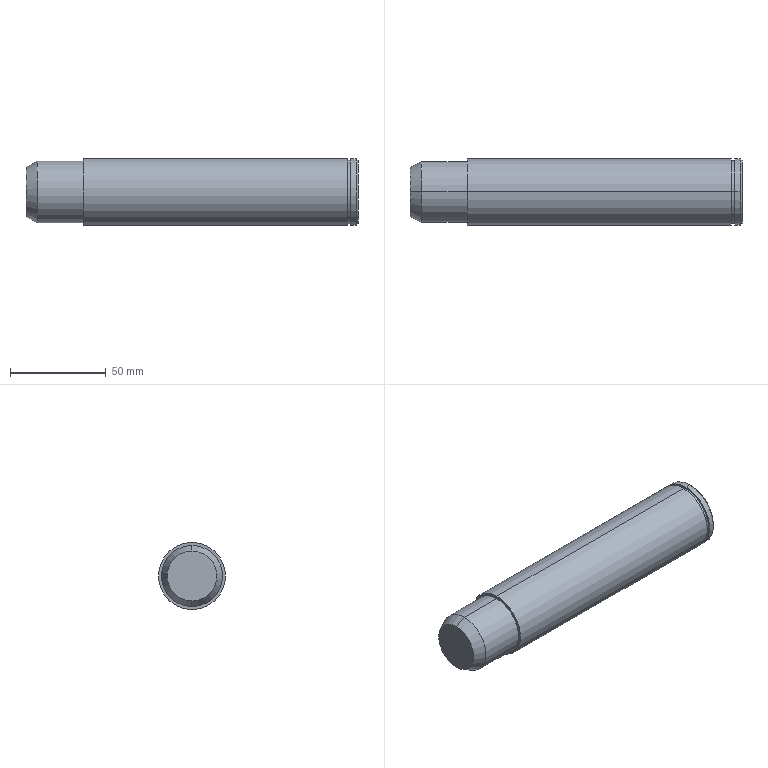Part | STEP file | 02-Support shaft 1 | 1 solid | 17 faces | box 173.5 x 35 x 35 mm | volume 161107 mm3 | cylinder 8 | plane 5 | cone 4 | commonest cylinder face diameters 35 x4 32 x2 33 x2
STEP:
#1=CARTESIAN_POINT('',(0.,0.,0.));
#2=DIRECTION('',(0.,0.,1.));
#3=DIRECTION('',(1.,0.,0.));
#4=AXIS2_PLACEMENT_3D('',#1,#2,#3);
#5=CARTESIAN_POINT('',(173.5,0.,16.5));
#6=VERTEX_POINT('',#5);
#7=CARTESIAN_POINT('',(173.5,0.,-16.5));
#8=VERTEX_POINT('',#7);
#9=CARTESIAN_POINT('',(173.5,0.,0.));
#10=DIRECTION('',(-1.,0.,0.));
#11=DIRECTION('',(0.,0.,1.));
#12=AXIS2_PLACEMENT_3D('',#9,#10,#11);
#13=CIRCLE('',#12,16.5);
#14=CARTESIAN_POINT('',(173.5,0.,0.));
#15=DIRECTION('',(-1.,0.,0.));
#16=DIRECTION('',(0.,0.,1.));
#17=AXIS2_PLACEMENT_3D('',#14,#15,#16);
#18=CONICAL_SURFACE('',#17,16.5,0.7854);
#19=CARTESIAN_POINT('',(0.,0.));
#20=DIRECTION('',(1.,0.));
#21=VECTOR('',#20,1.);
#22=LINE('',#19,#21);
#23=(GEOMETRIC_REPRESENTATION_CONTEXT(2)PARAMETRIC_REPRESENTATION_CONTEXT()REPRESENTATION_CONTEXT('',''));
#24=DEFINITIONAL_REPRESENTATION('',(#22),#23);
#25=PCURVE('',#18,#24);
#26=CARTESIAN_POINT('',(173.5,16.5,0.));
#27=DIRECTION('',(-1.,0.,0.));
#28=DIRECTION('',(0.,0.,1.));
#29=AXIS2_PLACEMENT_3D('',#26,#27,#28);
#30=PLANE('',#29);
#31=CARTESIAN_POINT('',(0.,-16.5));
#32=DIRECTION('',(1.,0.));
#33=AXIS2_PLACEMENT_2D('',#31,#32);
#34=CIRCLE('',#33,16.5);
#35=(GEOMETRIC_REPRESENTATION_CONTEXT(2)PARAMETRIC_REPRESENTATION_CONTEXT()REPRESENTATION_CONTEXT('',''));
#36=DEFINITIONAL_REPRESENTATION('',(#34),#35);
#37=PCURVE('',#30,#36);
#38=SURFACE_CURVE('',#13,(#25,#37),.PCURVE_S1.);
#39=EDGE_CURVE('',#6,#8,#38,.T.);
#40=ORIENTED_EDGE('',*,*,#39,.T.);
#41=CARTESIAN_POINT('',(172.5,0.,-17.5));
#42=VERTEX_POINT('',#41);
#43=CARTESIAN_POINT('',(173.5,0.,-16.5));
#44=DIRECTION('',(-0.7071,0.,-0.7071));
#45=VECTOR('',#44,1.);
#46=LINE('',#43,#45);
#47=CARTESIAN_POINT('',(3.142,0.));
#48=DIRECTION('',(0.,1.));
#49=VECTOR('',#48,1.);
#50=LINE('',#47,#49);
#51=(GEOMETRIC_REPRESENTATION_CONTEXT(2)PARAMETRIC_REPRESENTATION_CONTEXT()REPRESENTATION_CONTEXT('',''));
#52=DEFINITIONAL_REPRESENTATION('',(#50),#51);
#53=PCURVE('',#18,#52);
#54=CARTESIAN_POINT('',(173.5,0.,0.));
#55=DIRECTION('',(-1.,0.,0.));
#56=DIRECTION('',(0.,0.,1.));
#57=AXIS2_PLACEMENT_3D('',#54,#55,#56);
#58=CONICAL_SURFACE('',#57,16.5,0.7854);
#59=CARTESIAN_POINT('',(3.142,0.));
#60=DIRECTION('',(0.,1.));
#61=VECTOR('',#60,1.);
#62=LINE('',#59,#61);
#63=(GEOMETRIC_REPRESENTATION_CONTEXT(2)PARAMETRIC_REPRESENTATION_CONTEXT()REPRESENTATION_CONTEXT('',''));
#64=DEFINITIONAL_REPRESENTATION('',(#62),#63);
#65=PCURVE('',#58,#64);
#66=SURFACE_CURVE('',#46,(#53,#65),.PCURVE_S1.);
#67=EDGE_CURVE('',#8,#42,#66,.T.);
#68=ORIENTED_EDGE('',*,*,#67,.T.);
#69=CARTESIAN_POINT('',(172.5,0.,17.5));
#70=VERTEX_POINT('',#69);
#71=CARTESIAN_POINT('',(172.5,0.,0.));
#72=DIRECTION('',(-1.,0.,0.));
#73=DIRECTION('',(0.,0.,1.));
#74=AXIS2_PLACEMENT_3D('',#71,#72,#73);
#75=CIRCLE('',#74,17.5);
#76=CARTESIAN_POINT('',(0.,1.));
#77=DIRECTION('',(1.,0.));
#78=VECTOR('',#77,1.);
#79=LINE('',#76,#78);
#80=(GEOMETRIC_REPRESENTATION_CONTEXT(2)PARAMETRIC_REPRESENTATION_CONTEXT()REPRESENTATION_CONTEXT('',''));
#81=DEFINITIONAL_REPRESENTATION('',(#79),#80);
#82=PCURVE('',#18,#81);
#83=CARTESIAN_POINT('',(0.,0.,0.));
#84=DIRECTION('',(-1.,0.,0.));
#85=DIRECTION('',(0.,0.,1.));
#86=AXIS2_PLACEMENT_3D('',#83,#84,#85);
#87=CYLINDRICAL_SURFACE('',#86,17.5);
#88=CARTESIAN_POINT('',(0.,-172.5));
#89=DIRECTION('',(1.,0.));
#90=VECTOR('',#89,1.);
#91=LINE('',#88,#90);
#92=(GEOMETRIC_REPRESENTATION_CONTEXT(2)PARAMETRIC_REPRESENTATION_CONTEXT()REPRESENTATION_CONTEXT('',''));
#93=DEFINITIONAL_REPRESENTATION('',(#91),#92);
#94=PCURVE('',#87,#93);
#95=SURFACE_CURVE('',#75,(#82,#94),.PCURVE_S1.);
#96=EDGE_CURVE('',#70,#42,#95,.T.);
#97=ORIENTED_EDGE('',*,*,#96,.F.);
#98=CARTESIAN_POINT('',(173.5,0.,16.5));
#99=DIRECTION('',(-0.7071,0.,0.7071));
#100=VECTOR('',#99,1.);
#101=LINE('',#98,#100);
#102=CARTESIAN_POINT('',(0.,0.));
#103=DIRECTION('',(0.,1.));
#104=VECTOR('',#103,1.);
#105=LINE('',#102,#104);
#106=(GEOMETRIC_REPRESENTATION_CONTEXT(2)PARAMETRIC_REPRESENTATION_CONTEXT()REPRESENTATION_CONTEXT('',''));
#107=DEFINITIONAL_REPRESENTATION('',(#105),#106);
#108=PCURVE('',#18,#107);
#109=CARTESIAN_POINT('',(6.283,0.));
#110=DIRECTION('',(0.,1.));
#111=VECTOR('',#110,1.);
#112=LINE('',#109,#111);
#113=(GEOMETRIC_REPRESENTATION_CONTEXT(2)PARAMETRIC_REPRESENTATION_CONTEXT()REPRESENTATION_CONTEXT('',''));
#114=DEFINITIONAL_REPRESENTATION('',(#112),#113);
#115=PCURVE('',#58,#114);
#116=SURFACE_CURVE('',#101,(#108,#115),.PCURVE_S1.);
#117=EDGE_CURVE('',#6,#70,#116,.T.);
#118=ORIENTED_EDGE('',*,*,#117,.F.);
#119=EDGE_LOOP('',(#40,#68,#97,#118));
#120=FACE_BOUND('',#119,.T.);
#121=ADVANCED_FACE('',(#120),#18,.T.);
#122=ORIENTED_EDGE('',*,*,#96,.T.);
#123=CARTESIAN_POINT('',(169.7,0.,-17.5));
#124=VERTEX_POINT('',#123);
#125=CARTESIAN_POINT('',(0.,0.,-17.5));
#126=DIRECTION('',(-1.,0.,0.));
#127=VECTOR('',#126,1.);
#128=LINE('',#125,#127);
#129=CARTESIAN_POINT('',(3.142,0.));
#130=DIRECTION('',(0.,1.));
#131=VECTOR('',#130,1.);
#132=LINE('',#129,#131);
#133=(GEOMETRIC_REPRESENTATION_CONTEXT(2)PARAMETRIC_REPRESENTATION_CONTEXT()REPRESENTATION_CONTEXT('',''));
#134=DEFINITIONAL_REPRESENTATION('',(#132),#133);
#135=PCURVE('',#87,#134);
#136=CARTESIAN_POINT('',(0.,0.,0.));
#137=DIRECTION('',(-1.,0.,0.));
#138=DIRECTION('',(0.,0.,1.));
#139=AXIS2_PLACEMENT_3D('',#136,#137,#138);
#140=CYLINDRICAL_SURFACE('',#139,17.5);
#141=CARTESIAN_POINT('',(3.142,0.));
#142=DIRECTION('',(0.,1.));
#143=VECTOR('',#142,1.);
#144=LINE('',#141,#143);
#145=(GEOMETRIC_REPRESENTATION_CONTEXT(2)PARAMETRIC_REPRESENTATION_CONTEXT()REPRESENTATION_CONTEXT('',''));
#146=DEFINITIONAL_REPRESENTATION('',(#144),#145);
#147=PCURVE('',#140,#146);
#148=SURFACE_CURVE('',#128,(#135,#147),.PCURVE_S1.);
#149=EDGE_CURVE('',#42,#124,#148,.T.);
#150=ORIENTED_EDGE('',*,*,#149,.T.);
#151=CARTESIAN_POINT('',(169.7,0.,17.5));
#152=VERTEX_POINT('',#151);
#153=CARTESIAN_POINT('',(169.7,0.,0.));
#154=DIRECTION('',(-1.,0.,0.));
#155=DIRECTION('',(0.,0.,1.));
#156=AXIS2_PLACEMENT_3D('',#153,#154,#155);
#157=CIRCLE('',#156,17.5);
#158=CARTESIAN_POINT('',(0.,-169.7));
#159=DIRECTION('',(1.,0.));
#160=VECTOR('',#159,1.);
#161=LINE('',#158,#160);
#162=(GEOMETRIC_REPRESENTATION_CONTEXT(2)PARAMETRIC_REPRESENTATION_CONTEXT()REPRESENTATION_CONTEXT('',''));
#163=DEFINITIONAL_REPRESENTATION('',(#161),#162);
#164=PCURVE('',#87,#163);
#165=CARTESIAN_POINT('',(169.7,16.5,0.));
#166=DIRECTION('',(1.,0.,0.));
#167=DIRECTION('',(0.,0.,-1.));
#168=AXIS2_PLACEMENT_3D('',#165,#166,#167);
#169=PLANE('',#168);
#170=CARTESIAN_POINT('',(-17.5,-16.5));
#171=CARTESIAN_POINT('',(-17.5,13.811));
#172=CARTESIAN_POINT('',(8.75,-1.345));
#173=CARTESIAN_POINT('',(35.,-16.5));
#174=CARTESIAN_POINT('',(8.75,-31.655));
#175=CARTESIAN_POINT('',(-17.5,-46.811));
#176=CARTESIAN_POINT('',(-17.5,-16.5));
#177=(BOUNDED_CURVE()B_SPLINE_CURVE(2,(#170,#171,#172,#173,#174,#175,#176),.UNSPECIFIED.,.T.,.F.)B_SPLINE_CURVE_WITH_KNOTS((1,2,2,2,2,1),(-2.094,0.,2.094,4.189,6.283,8.378),.UNSPECIFIED.)CURVE()GEOMETRIC_REPRESENTATION_ITEM()RATIONAL_B_SPLINE_CURVE((1.,0.5,1.,0.5,1.,0.5,1.))REPRESENTATION_ITEM(''));
#178=(GEOMETRIC_REPRESENTATION_CONTEXT(2)PARAMETRIC_REPRESENTATION_CONTEXT()REPRESENTATION_CONTEXT('',''));
#179=DEFINITIONAL_REPRESENTATION('',(#177),#178);
#180=PCURVE('',#169,#179);
#181=SURFACE_CURVE('',#157,(#164,#180),.PCURVE_S1.);
#182=EDGE_CURVE('',#152,#124,#181,.T.);
#183=ORIENTED_EDGE('',*,*,#182,.F.);
#184=CARTESIAN_POINT('',(0.,0.,17.5));
#185=DIRECTION('',(-1.,0.,0.));
#186=VECTOR('',#185,1.);
#187=LINE('',#184,#186);
#188=CARTESIAN_POINT('',(0.,0.));
#189=DIRECTION('',(0.,1.));
#190=VECTOR('',#189,1.);
#191=LINE('',#188,#190);
#192=(GEOMETRIC_REPRESENTATION_CONTEXT(2)PARAMETRIC_REPRESENTATION_CONTEXT()REPRESENTATION_CONTEXT('',''));
#193=DEFINITIONAL_REPRESENTATION('',(#191),#192);
#194=PCURVE('',#87,#193);
#195=CARTESIAN_POINT('',(6.283,0.));
#196=DIRECTION('',(0.,1.));
#197=VECTOR('',#196,1.);
#198=LINE('',#195,#197);
#199=(GEOMETRIC_REPRESENTATION_CONTEXT(2)PARAMETRIC_REPRESENTATION_CONTEXT()REPRESENTATION_CONTEXT('',''));
#200=DEFINITIONAL_REPRESENTATION('',(#198),#199);
#201=PCURVE('',#140,#200);
#202=SURFACE_CURVE('',#187,(#194,#201),.PCURVE_S1.);
#203=EDGE_CURVE('',#70,#152,#202,.T.);
#204=ORIENTED_EDGE('',*,*,#203,.F.);
#205=EDGE_LOOP('',(#122,#150,#183,#204));
#206=FACE_BOUND('',#205,.T.);
#207=ADVANCED_FACE('',(#206),#87,.T.);
#208=CARTESIAN_POINT('',(169.7,0.,16.5));
#209=VERTEX_POINT('',#208);
#210=CARTESIAN_POINT('',(169.7,0.,-16.5));
#211=VERTEX_POINT('',#210);
#212=CARTESIAN_POINT('',(169.7,0.,0.));
#213=DIRECTION('',(-1.,0.,0.));
#214=DIRECTION('',(0.,0.,1.));
#215=AXIS2_PLACEMENT_3D('',#212,#213,#214);
#216=CIRCLE('',#215,16.5);
#217=CARTESIAN_POINT('',(0.,0.,0.));
#218=DIRECTION('',(-1.,0.,0.));
#219=DIRECTION('',(0.,0.,1.));
#220=AXIS2_PLACEMENT_3D('',#217,#218,#219);
#221=CYLINDRICAL_SURFACE('',#220,16.5);
#222=CARTESIAN_POINT('',(0.,-169.7));
#223=DIRECTION('',(1.,0.));
#224=VECTOR('',#223,1.);
#225=LINE('',#222,#224);
#226=(GEOMETRIC_REPRESENTATION_CONTEXT(2)PARAMETRIC_REPRESENTATION_CONTEXT()REPRESENTATION_CONTEXT('',''));
#227=DEFINITIONAL_REPRESENTATION('',(#225),#226);
#228=PCURVE('',#221,#227);
#229=CARTESIAN_POINT('',(-16.5,-16.5));
#230=CARTESIAN_POINT('',(-16.5,12.079));
#231=CARTESIAN_POINT('',(8.25,-2.211));
#232=CARTESIAN_POINT('',(33.,-16.5));
#233=CARTESIAN_POINT('',(8.25,-30.789));
#234=CARTESIAN_POINT('',(-16.5,-45.079));
#235=CARTESIAN_POINT('',(-16.5,-16.5));
#236=(BOUNDED_CURVE()B_SPLINE_CURVE(2,(#229,#230,#231,#232,#233,#234,#235),.UNSPECIFIED.,.T.,.F.)B_SPLINE_CURVE_WITH_KNOTS((1,2,2,2,2,1),(-2.094,0.,2.094,4.189,6.283,8.378),.UNSPECIFIED.)CURVE()GEOMETRIC_REPRESENTATION_ITEM()RATIONAL_B_SPLINE_CURVE((1.,0.5,1.,0.5,1.,0.5,1.))REPRESENTATION_ITEM(''));
#237=(GEOMETRIC_REPRESENTATION_CONTEXT(2)PARAMETRIC_REPRESENTATION_CONTEXT()REPRESENTATION_CONTEXT('',''));
#238=DEFINITIONAL_REPRESENTATION('',(#236),#237);
#239=PCURVE('',#169,#238);
#240=SURFACE_CURVE('',#216,(#228,#239),.PCURVE_S1.);
#241=EDGE_CURVE('',#209,#211,#240,.T.);
#242=ORIENTED_EDGE('',*,*,#241,.T.);
#243=CARTESIAN_POINT('',(168.,0.,-16.5));
#244=VERTEX_POINT('',#243);
#245=CARTESIAN_POINT('',(0.,0.,-16.5));
#246=DIRECTION('',(-1.,0.,0.));
#247=VECTOR('',#246,1.);
#248=LINE('',#245,#247);
#249=CARTESIAN_POINT('',(3.142,0.));
#250=DIRECTION('',(0.,1.));
#251=VECTOR('',#250,1.);
#252=LINE('',#249,#251);
#253=(GEOMETRIC_REPRESENTATION_CONTEXT(2)PARAMETRIC_REPRESENTATION_CONTEXT()REPRESENTATION_CONTEXT('',''));
#254=DEFINITIONAL_REPRESENTATION('',(#252),#253);
#255=PCURVE('',#221,#254);
#256=CARTESIAN_POINT('',(0.,0.,0.));
#257=DIRECTION('',(-1.,0.,0.));
#258=DIRECTION('',(0.,0.,1.));
#259=AXIS2_PLACEMENT_3D('',#256,#257,#258);
#260=CYLINDRICAL_SURFACE('',#259,16.5);
#261=CARTESIAN_POINT('',(3.142,0.));
#262=DIRECTION('',(0.,1.));
#263=VECTOR('',#262,1.);
#264=LINE('',#261,#263);
#265=(GEOMETRIC_REPRESENTATION_CONTEXT(2)PARAMETRIC_REPRESENTATION_CONTEXT()REPRESENTATION_CONTEXT('',''));
#266=DEFINITIONAL_REPRESENTATION('',(#264),#265);
#267=PCURVE('',#260,#266);
#268=SURFACE_CURVE('',#248,(#255,#267),.PCURVE_S1.);
#269=EDGE_CURVE('',#211,#244,#268,.T.);
#270=ORIENTED_EDGE('',*,*,#269,.T.);
#271=CARTESIAN_POINT('',(168.,0.,16.5));
#272=VERTEX_POINT('',#271);
#273=CARTESIAN_POINT('',(168.,0.,0.));
#274=DIRECTION('',(-1.,0.,0.));
#275=DIRECTION('',(0.,0.,1.));
#276=AXIS2_PLACEMENT_3D('',#273,#274,#275);
#277=CIRCLE('',#276,16.5);
#278=CARTESIAN_POINT('',(0.,-168.));
#279=DIRECTION('',(1.,0.));
#280=VECTOR('',#279,1.);
#281=LINE('',#278,#280);
#282=(GEOMETRIC_REPRESENTATION_CONTEXT(2)PARAMETRIC_REPRESENTATION_CONTEXT()REPRESENTATION_CONTEXT('',''));
#283=DEFINITIONAL_REPRESENTATION('',(#281),#282);
#284=PCURVE('',#221,#283);
#285=CARTESIAN_POINT('',(168.,17.5,0.));
#286=DIRECTION('',(-1.,0.,0.));
#287=DIRECTION('',(0.,0.,1.));
#288=AXIS2_PLACEMENT_3D('',#285,#286,#287);
#289=PLANE('',#288);
#290=CARTESIAN_POINT('',(0.,-17.5));
#291=DIRECTION('',(1.,0.));
#292=AXIS2_PLACEMENT_2D('',#290,#291);
#293=CIRCLE('',#292,16.5);
#294=(GEOMETRIC_REPRESENTATION_CONTEXT(2)PARAMETRIC_REPRESENTATION_CONTEXT()REPRESENTATION_CONTEXT('',''));
#295=DEFINITIONAL_REPRESENTATION('',(#293),#294);
#296=PCURVE('',#289,#295);
#297=SURFACE_CURVE('',#277,(#284,#296),.PCURVE_S1.);
#298=EDGE_CURVE('',#272,#244,#297,.T.);
#299=ORIENTED_EDGE('',*,*,#298,.F.);
#300=CARTESIAN_POINT('',(0.,0.,16.5));
#301=DIRECTION('',(-1.,0.,0.));
#302=VECTOR('',#301,1.);
#303=LINE('',#300,#302);
#304=CARTESIAN_POINT('',(0.,0.));
#305=DIRECTION('',(0.,1.));
#306=VECTOR('',#305,1.);
#307=LINE('',#304,#306);
#308=(GEOMETRIC_REPRESENTATION_CONTEXT(2)PARAMETRIC_REPRESENTATION_CONTEXT()REPRESENTATION_CONTEXT('',''));
#309=DEFINITIONAL_REPRESENTATION('',(#307),#308);
#310=PCURVE('',#221,#309);
#311=CARTESIAN_POINT('',(6.283,0.));
#312=DIRECTION('',(0.,1.));
#313=VECTOR('',#312,1.);
#314=LINE('',#311,#313);
#315=(GEOMETRIC_REPRESENTATION_CONTEXT(2)PARAMETRIC_REPRESENTATION_CONTEXT()REPRESENTATION_CONTEXT('',''));
#316=DEFINITIONAL_REPRESENTATION('',(#314),#315);
#317=PCURVE('',#260,#316);
#318=SURFACE_CURVE('',#303,(#310,#317),.PCURVE_S1.);
#319=EDGE_CURVE('',#209,#272,#318,.T.);
#320=ORIENTED_EDGE('',*,*,#319,.F.);
#321=EDGE_LOOP('',(#242,#270,#299,#320));
#322=FACE_BOUND('',#321,.T.);
#323=ADVANCED_FACE('',(#322),#221,.T.);
#324=CARTESIAN_POINT('',(168.,0.,17.5));
#325=VERTEX_POINT('',#324);
#326=CARTESIAN_POINT('',(168.,0.,-17.5));
#327=VERTEX_POINT('',#326);
#328=CARTESIAN_POINT('',(168.,0.,0.));
#329=DIRECTION('',(-1.,0.,0.));
#330=DIRECTION('',(0.,0.,1.));
#331=AXIS2_PLACEMENT_3D('',#328,#329,#330);
#332=CIRCLE('',#331,17.5);
#333=CARTESIAN_POINT('',(0.,0.,0.));
#334=DIRECTION('',(-1.,0.,0.));
#335=DIRECTION('',(0.,0.,1.));
#336=AXIS2_PLACEMENT_3D('',#333,#334,#335);
#337=CYLINDRICAL_SURFACE('',#336,17.5);
#338=CARTESIAN_POINT('',(0.,-168.));
#339=DIRECTION('',(1.,0.));
#340=VECTOR('',#339,1.);
#341=LINE('',#338,#340);
#342=(GEOMETRIC_REPRESENTATION_CONTEXT(2)PARAMETRIC_REPRESENTATION_CONTEXT()REPRESENTATION_CONTEXT('',''));
#343=DEFINITIONAL_REPRESENTATION('',(#341),#342);
#344=PCURVE('',#337,#343);
#345=CARTESIAN_POINT('',(0.,-17.5));
#346=DIRECTION('',(1.,0.));
#347=AXIS2_PLACEMENT_2D('',#345,#346);
#348=CIRCLE('',#347,17.5);
#349=(GEOMETRIC_REPRESENTATION_CONTEXT(2)PARAMETRIC_REPRESENTATION_CONTEXT()REPRESENTATION_CONTEXT('',''));
#350=DEFINITIONAL_REPRESENTATION('',(#348),#349);
#351=PCURVE('',#289,#350);
#352=SURFACE_CURVE('',#332,(#344,#351),.PCURVE_S1.);
#353=EDGE_CURVE('',#325,#327,#352,.T.);
#354=ORIENTED_EDGE('',*,*,#353,.T.);
#355=CARTESIAN_POINT('',(30.,0.,-17.5));
#356=VERTEX_POINT('',#355);
#357=CARTESIAN_POINT('',(0.,0.,-17.5));
#358=DIRECTION('',(-1.,0.,0.));
#359=VECTOR('',#358,1.);
#360=LINE('',#357,#359);
#361=CARTESIAN_POINT('',(3.142,0.));
#362=DIRECTION('',(0.,1.));
#363=VECTOR('',#362,1.);
#364=LINE('',#361,#363);
#365=(GEOMETRIC_REPRESENTATION_CONTEXT(2)PARAMETRIC_REPRESENTATION_CONTEXT()REPRESENTATION_CONTEXT('',''));
#366=DEFINITIONAL_REPRESENTATION('',(#364),#365);
#367=PCURVE('',#337,#366);
#368=CARTESIAN_POINT('',(0.,0.,0.));
#369=DIRECTION('',(-1.,0.,0.));
#370=DIRECTION('',(0.,0.,1.));
#371=AXIS2_PLACEMENT_3D('',#368,#369,#370);
#372=CYLINDRICAL_SURFACE('',#371,17.5);
#373=CARTESIAN_POINT('',(3.142,0.));
#374=DIRECTION('',(0.,1.));
#375=VECTOR('',#374,1.);
#376=LINE('',#373,#375);
#377=(GEOMETRIC_REPRESENTATION_CONTEXT(2)PARAMETRIC_REPRESENTATION_CONTEXT()REPRESENTATION_CONTEXT('',''));
#378=DEFINITIONAL_REPRESENTATION('',(#376),#377);
#379=PCURVE('',#372,#378);
#380=SURFACE_CURVE('',#360,(#367,#379),.PCURVE_S1.);
#381=EDGE_CURVE('',#327,#356,#380,.T.);
#382=ORIENTED_EDGE('',*,*,#381,.T.);
#383=CARTESIAN_POINT('',(30.,0.,17.5));
#384=VERTEX_POINT('',#383);
#385=CARTESIAN_POINT('',(30.,0.,0.));
#386=DIRECTION('',(-1.,0.,0.));
#387=DIRECTION('',(0.,0.,1.));
#388=AXIS2_PLACEMENT_3D('',#385,#386,#387);
#389=CIRCLE('',#388,17.5);
#390=CARTESIAN_POINT('',(0.,-30.));
#391=DIRECTION('',(1.,0.));
#392=VECTOR('',#391,1.);
#393=LINE('',#390,#392);
#394=(GEOMETRIC_REPRESENTATION_CONTEXT(2)PARAMETRIC_REPRESENTATION_CONTEXT()REPRESENTATION_CONTEXT('',''));
#395=DEFINITIONAL_REPRESENTATION('',(#393),#394);
#396=PCURVE('',#337,#395);
#397=CARTESIAN_POINT('',(30.,16.,0.));
#398=DIRECTION('',(1.,0.,0.));
#399=DIRECTION('',(0.,0.,-1.));
#400=AXIS2_PLACEMENT_3D('',#397,#398,#399);
#401=PLANE('',#400);
#402=CARTESIAN_POINT('',(-17.5,-16.));
#403=CARTESIAN_POINT('',(-17.5,14.311));
#404=CARTESIAN_POINT('',(8.75,-0.8446));
#405=CARTESIAN_POINT('',(35.,-16.));
#406=CARTESIAN_POINT('',(8.75,-31.155));
#407=CARTESIAN_POINT('',(-17.5,-46.311));
#408=CARTESIAN_POINT('',(-17.5,-16.));
#409=(BOUNDED_CURVE()B_SPLINE_CURVE(2,(#402,#403,#404,#405,#406,#407,#408),.UNSPECIFIED.,.T.,.F.)B_SPLINE_CURVE_WITH_KNOTS((1,2,2,2,2,1),(-2.094,0.,2.094,4.189,6.283,8.378),.UNSPECIFIED.)CURVE()GEOMETRIC_REPRESENTATION_ITEM()RATIONAL_B_SPLINE_CURVE((1.,0.5,1.,0.5,1.,0.5,1.))REPRESENTATION_ITEM(''));
#410=(GEOMETRIC_REPRESENTATION_CONTEXT(2)PARAMETRIC_REPRESENTATION_CONTEXT()REPRESENTATION_CONTEXT('',''));
#411=DEFINITIONAL_REPRESENTATION('',(#409),#410);
#412=PCURVE('',#401,#411);
#413=SURFACE_CURVE('',#389,(#396,#412),.PCURVE_S1.);
#414=EDGE_CURVE('',#384,#356,#413,.T.);
#415=ORIENTED_EDGE('',*,*,#414,.F.);
#416=CARTESIAN_POINT('',(0.,0.,17.5));
#417=DIRECTION('',(-1.,0.,0.));
#418=VECTOR('',#417,1.);
#419=LINE('',#416,#418);
#420=CARTESIAN_POINT('',(0.,0.));
#421=DIRECTION('',(0.,1.));
#422=VECTOR('',#421,1.);
#423=LINE('',#420,#422);
#424=(GEOMETRIC_REPRESENTATION_CONTEXT(2)PARAMETRIC_REPRESENTATION_CONTEXT()REPRESENTATION_CONTEXT('',''));
#425=DEFINITIONAL_REPRESENTATION('',(#423),#424);
#426=PCURVE('',#337,#425);
#427=CARTESIAN_POINT('',(6.283,0.));
#428=DIRECTION('',(0.,1.));
#429=VECTOR('',#428,1.);
#430=LINE('',#427,#429);
#431=(GEOMETRIC_REPRESENTATION_CONTEXT(2)PARAMETRIC_REPRESENTATION_CONTEXT()REPRESENTATION_CONTEXT('',''));
#432=DEFINITIONAL_REPRESENTATION('',(#430),#431);
#433=PCURVE('',#372,#432);
#434=SURFACE_CURVE('',#419,(#426,#433),.PCURVE_S1.);
#435=EDGE_CURVE('',#325,#384,#434,.T.);
#436=ORIENTED_EDGE('',*,*,#435,.F.);
#437=EDGE_LOOP('',(#354,#382,#415,#436));
#438=FACE_BOUND('',#437,.T.);
#439=ADVANCED_FACE('',(#438),#337,.T.);
#440=CARTESIAN_POINT('',(30.,0.,16.));
#441=VERTEX_POINT('',#440);
#442=CARTESIAN_POINT('',(30.,0.,-16.));
#443=VERTEX_POINT('',#442);
#444=CARTESIAN_POINT('',(30.,0.,0.));
#445=DIRECTION('',(-1.,0.,0.));
#446=DIRECTION('',(0.,0.,1.));
#447=AXIS2_PLACEMENT_3D('',#444,#445,#446);
#448=CIRCLE('',#447,16.);
#449=CARTESIAN_POINT('',(0.,0.,0.));
#450=DIRECTION('',(-1.,0.,0.));
#451=DIRECTION('',(0.,0.,1.));
#452=AXIS2_PLACEMENT_3D('',#449,#450,#451);
#453=CYLINDRICAL_SURFACE('',#452,16.);
#454=CARTESIAN_POINT('',(0.,-30.));
#455=DIRECTION('',(1.,0.));
#456=VECTOR('',#455,1.);
#457=LINE('',#454,#456);
#458=(GEOMETRIC_REPRESENTATION_CONTEXT(2)PARAMETRIC_REPRESENTATION_CONTEXT()REPRESENTATION_CONTEXT('',''));
#459=DEFINITIONAL_REPRESENTATION('',(#457),#458);
#460=PCURVE('',#453,#459);
#461=CARTESIAN_POINT('',(-16.,-16.));
#462=CARTESIAN_POINT('',(-16.,11.713));
#463=CARTESIAN_POINT('',(8.,-2.144));
#464=CARTESIAN_POINT('',(32.,-16.));
#465=CARTESIAN_POINT('',(8.,-29.856));
#466=CARTESIAN_POINT('',(-16.,-43.713));
#467=CARTESIAN_POINT('',(-16.,-16.));
#468=(BOUNDED_CURVE()B_SPLINE_CURVE(2,(#461,#462,#463,#464,#465,#466,#467),.UNSPECIFIED.,.T.,.F.)B_SPLINE_CURVE_WITH_KNOTS((1,2,2,2,2,1),(-2.094,0.,2.094,4.189,6.283,8.378),.UNSPECIFIED.)CURVE()GEOMETRIC_REPRESENTATION_ITEM()RATIONAL_B_SPLINE_CURVE((1.,0.5,1.,0.5,1.,0.5,1.))REPRESENTATION_ITEM(''));
#469=(GEOMETRIC_REPRESENTATION_CONTEXT(2)PARAMETRIC_REPRESENTATION_CONTEXT()REPRESENTATION_CONTEXT('',''));
#470=DEFINITIONAL_REPRESENTATION('',(#468),#469);
#471=PCURVE('',#401,#470);
#472=SURFACE_CURVE('',#448,(#460,#471),.PCURVE_S1.);
#473=EDGE_CURVE('',#441,#443,#472,.T.);
#474=ORIENTED_EDGE('',*,*,#473,.T.);
#475=CARTESIAN_POINT('',(6.,0.,-16.));
#476=VERTEX_POINT('',#475);
#477=CARTESIAN_POINT('',(0.,0.,-16.));
#478=DIRECTION('',(-1.,0.,0.));
#479=VECTOR('',#478,1.);
#480=LINE('',#477,#479);
#481=CARTESIAN_POINT('',(3.142,0.));
#482=DIRECTION('',(0.,1.));
#483=VECTOR('',#482,1.);
#484=LINE('',#481,#483);
#485=(GEOMETRIC_REPRESENTATION_CONTEXT(2)PARAMETRIC_REPRESENTATION_CONTEXT()REPRESENTATION_CONTEXT('',''));
#486=DEFINITIONAL_REPRESENTATION('',(#484),#485);
#487=PCURVE('',#453,#486);
#488=CARTESIAN_POINT('',(0.,0.,0.));
#489=DIRECTION('',(-1.,0.,0.));
#490=DIRECTION('',(0.,0.,1.));
#491=AXIS2_PLACEMENT_3D('',#488,#489,#490);
#492=CYLINDRICAL_SURFACE('',#491,16.);
#493=CARTESIAN_POINT('',(3.142,0.));
#494=DIRECTION('',(0.,1.));
#495=VECTOR('',#494,1.);
#496=LINE('',#493,#495);
#497=(GEOMETRIC_REPRESENTATION_CONTEXT(2)PARAMETRIC_REPRESENTATION_CONTEXT()REPRESENTATION_CONTEXT('',''));
#498=DEFINITIONAL_REPRESENTATION('',(#496),#497);
#499=PCURVE('',#492,#498);
#500=SURFACE_CURVE('',#480,(#487,#499),.PCURVE_S1.);
#501=EDGE_CURVE('',#443,#476,#500,.T.);
#502=ORIENTED_EDGE('',*,*,#501,.T.);
#503=CARTESIAN_POINT('',(6.,0.,16.));
#504=VERTEX_POINT('',#503);
#505=CARTESIAN_POINT('',(6.,0.,0.));
#506=DIRECTION('',(-1.,0.,0.));
#507=DIRECTION('',(0.,0.,1.));
#508=AXIS2_PLACEMENT_3D('',#505,#506,#507);
#509=CIRCLE('',#508,16.);
#510=CARTESIAN_POINT('',(0.,-6.));
#511=DIRECTION('',(1.,0.));
#512=VECTOR('',#511,1.);
#513=LINE('',#510,#512);
#514=(GEOMETRIC_REPRESENTATION_CONTEXT(2)PARAMETRIC_REPRESENTATION_CONTEXT()REPRESENTATION_CONTEXT('',''));
#515=DEFINITIONAL_REPRESENTATION('',(#513),#514);
#516=PCURVE('',#453,#515);
#517=CARTESIAN_POINT('',(6.,0.,0.));
#518=DIRECTION('',(1.,0.,0.));
#519=DIRECTION('',(0.,0.,-1.));
#520=AXIS2_PLACEMENT_3D('',#517,#518,#519);
#521=CONICAL_SURFACE('',#520,16.,0.4636);
#522=CARTESIAN_POINT('',(3.142,0.));
#523=DIRECTION('',(-1.,0.));
#524=VECTOR('',#523,1.);
#525=LINE('',#522,#524);
#526=(GEOMETRIC_REPRESENTATION_CONTEXT(2)PARAMETRIC_REPRESENTATION_CONTEXT()REPRESENTATION_CONTEXT('',''));
#527=DEFINITIONAL_REPRESENTATION('',(#525),#526);
#528=PCURVE('',#521,#527);
#529=SURFACE_CURVE('',#509,(#516,#528),.PCURVE_S1.);
#530=EDGE_CURVE('',#504,#476,#529,.T.);
#531=ORIENTED_EDGE('',*,*,#530,.F.);
#532=CARTESIAN_POINT('',(0.,0.,16.));
#533=DIRECTION('',(-1.,0.,0.));
#534=VECTOR('',#533,1.);
#535=LINE('',#532,#534);
#536=CARTESIAN_POINT('',(0.,0.));
#537=DIRECTION('',(0.,1.));
#538=VECTOR('',#537,1.);
#539=LINE('',#536,#538);
#540=(GEOMETRIC_REPRESENTATION_CONTEXT(2)PARAMETRIC_REPRESENTATION_CONTEXT()REPRESENTATION_CONTEXT('',''));
#541=DEFINITIONAL_REPRESENTATION('',(#539),#540);
#542=PCURVE('',#453,#541);
#543=CARTESIAN_POINT('',(6.283,0.));
#544=DIRECTION('',(0.,1.));
#545=VECTOR('',#544,1.);
#546=LINE('',#543,#545);
#547=(GEOMETRIC_REPRESENTATION_CONTEXT(2)PARAMETRIC_REPRESENTATION_CONTEXT()REPRESENTATION_CONTEXT('',''));
#548=DEFINITIONAL_REPRESENTATION('',(#546),#547);
#549=PCURVE('',#492,#548);
#550=SURFACE_CURVE('',#535,(#542,#549),.PCURVE_S1.);
#551=EDGE_CURVE('',#441,#504,#550,.T.);
#552=ORIENTED_EDGE('',*,*,#551,.F.);
#553=EDGE_LOOP('',(#474,#502,#531,#552));
#554=FACE_BOUND('',#553,.T.);
#555=ADVANCED_FACE('',(#554),#453,.T.);
#556=CARTESIAN_POINT('',(0.,0.,13.));
#557=VERTEX_POINT('',#556);
#558=CARTESIAN_POINT('',(0.,0.,-13.));
#559=VERTEX_POINT('',#558);
#560=CARTESIAN_POINT('',(0.,0.,0.));
#561=DIRECTION('',(-1.,0.,0.));
#562=DIRECTION('',(0.,0.,1.));
#563=AXIS2_PLACEMENT_3D('',#560,#561,#562);
#564=CIRCLE('',#563,13.);
#565=CARTESIAN_POINT('',(3.142,-6.));
#566=DIRECTION('',(-1.,0.));
#567=VECTOR('',#566,1.);
#568=LINE('',#565,#567);
#569=(GEOMETRIC_REPRESENTATION_CONTEXT(2)PARAMETRIC_REPRESENTATION_CONTEXT()REPRESENTATION_CONTEXT('',''));
#570=DEFINITIONAL_REPRESENTATION('',(#568),#569);
#571=PCURVE('',#521,#570);
#572=CARTESIAN_POINT('',(0.,0.,0.));
#573=DIRECTION('',(1.,0.,0.));
#574=DIRECTION('',(0.,0.,-1.));
#575=AXIS2_PLACEMENT_3D('',#572,#573,#574);
#576=PLANE('',#575);
#577=CARTESIAN_POINT('',(-13.,0.));
#578=CARTESIAN_POINT('',(-13.,22.517));
#579=CARTESIAN_POINT('',(6.5,11.258));
#580=CARTESIAN_POINT('',(26.,0.));
#581=CARTESIAN_POINT('',(6.5,-11.258));
#582=CARTESIAN_POINT('',(-13.,-22.517));
#583=CARTESIAN_POINT('',(-13.,0.));
#584=(BOUNDED_CURVE()B_SPLINE_CURVE(2,(#577,#578,#579,#580,#581,#582,#583),.UNSPECIFIED.,.T.,.F.)B_SPLINE_CURVE_WITH_KNOTS((1,2,2,2,2,1),(-2.094,0.,2.094,4.189,6.283,8.378),.UNSPECIFIED.)CURVE()GEOMETRIC_REPRESENTATION_ITEM()RATIONAL_B_SPLINE_CURVE((1.,0.5,1.,0.5,1.,0.5,1.))REPRESENTATION_ITEM(''));
#585=(GEOMETRIC_REPRESENTATION_CONTEXT(2)PARAMETRIC_REPRESENTATION_CONTEXT()REPRESENTATION_CONTEXT('',''));
#586=DEFINITIONAL_REPRESENTATION('',(#584),#585);
#587=PCURVE('',#576,#586);
#588=SURFACE_CURVE('',#564,(#571,#587),.PCURVE_S1.);
#589=EDGE_CURVE('',#557,#559,#588,.T.);
#590=ORIENTED_EDGE('',*,*,#589,.F.);
#591=CARTESIAN_POINT('',(6.,0.,16.));
#592=DIRECTION('',(0.8944,0.,0.4472));
#593=VECTOR('',#592,1.);
#594=LINE('',#591,#593);
#595=CARTESIAN_POINT('',(3.142,0.));
#596=DIRECTION('',(0.,1.));
#597=VECTOR('',#596,1.);
#598=LINE('',#595,#597);
#599=(GEOMETRIC_REPRESENTATION_CONTEXT(2)PARAMETRIC_REPRESENTATION_CONTEXT()REPRESENTATION_CONTEXT('',''));
#600=DEFINITIONAL_REPRESENTATION('',(#598),#599);
#601=PCURVE('',#521,#600);
#602=CARTESIAN_POINT('',(6.,0.,0.));
#603=DIRECTION('',(1.,0.,0.));
#604=DIRECTION('',(0.,0.,-1.));
#605=AXIS2_PLACEMENT_3D('',#602,#603,#604);
#606=CONICAL_SURFACE('',#605,16.,0.4636);
#607=CARTESIAN_POINT('',(3.142,0.));
#608=DIRECTION('',(0.,1.));
#609=VECTOR('',#608,1.);
#610=LINE('',#607,#609);
#611=(GEOMETRIC_REPRESENTATION_CONTEXT(2)PARAMETRIC_REPRESENTATION_CONTEXT()REPRESENTATION_CONTEXT('',''));
#612=DEFINITIONAL_REPRESENTATION('',(#610),#611);
#613=PCURVE('',#606,#612);
#614=SURFACE_CURVE('',#594,(#601,#613),.PCURVE_S1.);
#615=EDGE_CURVE('',#557,#504,#614,.T.);
#616=ORIENTED_EDGE('',*,*,#615,.T.);
#617=ORIENTED_EDGE('',*,*,#530,.T.);
#618=CARTESIAN_POINT('',(6.,0.,-16.));
#619=DIRECTION('',(0.8944,0.,-0.4472));
#620=VECTOR('',#619,1.);
#621=LINE('',#618,#620);
#622=CARTESIAN_POINT('',(0.,0.));
#623=DIRECTION('',(0.,1.));
#624=VECTOR('',#623,1.);
#625=LINE('',#622,#624);
#626=(GEOMETRIC_REPRESENTATION_CONTEXT(2)PARAMETRIC_REPRESENTATION_CONTEXT()REPRESENTATION_CONTEXT('',''));
#627=DEFINITIONAL_REPRESENTATION('',(#625),#626);
#628=PCURVE('',#521,#627);
#629=CARTESIAN_POINT('',(6.283,0.));
#630=DIRECTION('',(0.,1.));
#631=VECTOR('',#630,1.);
#632=LINE('',#629,#631);
#633=(GEOMETRIC_REPRESENTATION_CONTEXT(2)PARAMETRIC_REPRESENTATION_CONTEXT()REPRESENTATION_CONTEXT('',''));
#634=DEFINITIONAL_REPRESENTATION('',(#632),#633);
#635=PCURVE('',#606,#634);
#636=SURFACE_CURVE('',#621,(#628,#635),.PCURVE_S1.);
#637=EDGE_CURVE('',#559,#476,#636,.T.);
#638=ORIENTED_EDGE('',*,*,#637,.F.);
#639=EDGE_LOOP('',(#590,#616,#617,#638));
#640=FACE_BOUND('',#639,.T.);
#641=ADVANCED_FACE('',(#640),#521,.T.);
#642=CARTESIAN_POINT('',(0.,0.,0.));
#643=DIRECTION('',(-1.,0.,0.));
#644=DIRECTION('',(0.,0.,1.));
#645=AXIS2_PLACEMENT_3D('',#642,#643,#644);
#646=CIRCLE('',#645,13.);
#647=CARTESIAN_POINT('',(-13.,0.));
#648=CARTESIAN_POINT('',(-13.,22.517));
#649=CARTESIAN_POINT('',(6.5,11.258));
#650=CARTESIAN_POINT('',(26.,0.));
#651=CARTESIAN_POINT('',(6.5,-11.258));
#652=CARTESIAN_POINT('',(-13.,-22.517));
#653=CARTESIAN_POINT('',(-13.,0.));
#654=(BOUNDED_CURVE()B_SPLINE_CURVE(2,(#647,#648,#649,#650,#651,#652,#653),.UNSPECIFIED.,.T.,.F.)B_SPLINE_CURVE_WITH_KNOTS((1,2,2,2,2,1),(-2.094,0.,2.094,4.189,6.283,8.378),.UNSPECIFIED.)CURVE()GEOMETRIC_REPRESENTATION_ITEM()RATIONAL_B_SPLINE_CURVE((1.,0.5,1.,0.5,1.,0.5,1.))REPRESENTATION_ITEM(''));
#655=(GEOMETRIC_REPRESENTATION_CONTEXT(2)PARAMETRIC_REPRESENTATION_CONTEXT()REPRESENTATION_CONTEXT('',''));
#656=DEFINITIONAL_REPRESENTATION('',(#654),#655);
#657=PCURVE('',#576,#656);
#658=CARTESIAN_POINT('',(9.425,-6.));
#659=DIRECTION('',(-1.,0.));
#660=VECTOR('',#659,1.);
#661=LINE('',#658,#660);
#662=(GEOMETRIC_REPRESENTATION_CONTEXT(2)PARAMETRIC_REPRESENTATION_CONTEXT()REPRESENTATION_CONTEXT('',''));
#663=DEFINITIONAL_REPRESENTATION('',(#661),#662);
#664=PCURVE('',#606,#663);
#665=SURFACE_CURVE('',#646,(#657,#664),.PCURVE_S1.);
#666=EDGE_CURVE('',#559,#557,#665,.T.);
#667=ORIENTED_EDGE('',*,*,#666,.T.);
#668=ORIENTED_EDGE('',*,*,#589,.T.);
#669=EDGE_LOOP('',(#667,#668));
#670=FACE_BOUND('',#669,.T.);
#671=ADVANCED_FACE('',(#670),#576,.F.);
#672=ORIENTED_EDGE('',*,*,#615,.F.);
#673=ORIENTED_EDGE('',*,*,#666,.F.);
#674=ORIENTED_EDGE('',*,*,#637,.T.);
#675=CARTESIAN_POINT('',(6.,0.,0.));
#676=DIRECTION('',(-1.,0.,0.));
#677=DIRECTION('',(0.,0.,1.));
#678=AXIS2_PLACEMENT_3D('',#675,#676,#677);
#679=CIRCLE('',#678,16.);
#680=CARTESIAN_POINT('',(9.425,0.));
#681=DIRECTION('',(-1.,0.));
#682=VECTOR('',#681,1.);
#683=LINE('',#680,#682);
#684=(GEOMETRIC_REPRESENTATION_CONTEXT(2)PARAMETRIC_REPRESENTATION_CONTEXT()REPRESENTATION_CONTEXT('',''));
#685=DEFINITIONAL_REPRESENTATION('',(#683),#684);
#686=PCURVE('',#606,#685);
#687=CARTESIAN_POINT('',(0.,-6.));
#688=DIRECTION('',(1.,0.));
#689=VECTOR('',#688,1.);
#690=LINE('',#687,#689);
#691=(GEOMETRIC_REPRESENTATION_CONTEXT(2)PARAMETRIC_REPRESENTATION_CONTEXT()REPRESENTATION_CONTEXT('',''));
#692=DEFINITIONAL_REPRESENTATION('',(#690),#691);
#693=PCURVE('',#492,#692);
#694=SURFACE_CURVE('',#679,(#686,#693),.PCURVE_S1.);
#695=EDGE_CURVE('',#476,#504,#694,.T.);
#696=ORIENTED_EDGE('',*,*,#695,.T.);
#697=EDGE_LOOP('',(#672,#673,#674,#696));
#698=FACE_BOUND('',#697,.T.);
#699=ADVANCED_FACE('',(#698),#606,.T.);
#700=ORIENTED_EDGE('',*,*,#501,.F.);
#701=CARTESIAN_POINT('',(30.,0.,0.));
#702=DIRECTION('',(-1.,0.,0.));
#703=DIRECTION('',(0.,0.,1.));
#704=AXIS2_PLACEMENT_3D('',#701,#702,#703);
#705=CIRCLE('',#704,16.);
#706=CARTESIAN_POINT('',(0.,-30.));
#707=DIRECTION('',(1.,0.));
#708=VECTOR('',#707,1.);
#709=LINE('',#706,#708);
#710=(GEOMETRIC_REPRESENTATION_CONTEXT(2)PARAMETRIC_REPRESENTATION_CONTEXT()REPRESENTATION_CONTEXT('',''));
#711=DEFINITIONAL_REPRESENTATION('',(#709),#710);
#712=PCURVE('',#492,#711);
#713=CARTESIAN_POINT('',(-16.,-16.));
#714=CARTESIAN_POINT('',(-16.,11.713));
#715=CARTESIAN_POINT('',(8.,-2.144));
#716=CARTESIAN_POINT('',(32.,-16.));
#717=CARTESIAN_POINT('',(8.,-29.856));
#718=CARTESIAN_POINT('',(-16.,-43.713));
#719=CARTESIAN_POINT('',(-16.,-16.));
#720=(BOUNDED_CURVE()B_SPLINE_CURVE(2,(#713,#714,#715,#716,#717,#718,#719),.UNSPECIFIED.,.T.,.F.)B_SPLINE_CURVE_WITH_KNOTS((1,2,2,2,2,1),(-2.094,0.,2.094,4.189,6.283,8.378),.UNSPECIFIED.)CURVE()GEOMETRIC_REPRESENTATION_ITEM()RATIONAL_B_SPLINE_CURVE((1.,0.5,1.,0.5,1.,0.5,1.))REPRESENTATION_ITEM(''));
#721=(GEOMETRIC_REPRESENTATION_CONTEXT(2)PARAMETRIC_REPRESENTATION_CONTEXT()REPRESENTATION_CONTEXT('',''));
#722=DEFINITIONAL_REPRESENTATION('',(#720),#721);
#723=PCURVE('',#401,#722);
#724=SURFACE_CURVE('',#705,(#712,#723),.PCURVE_S1.);
#725=EDGE_CURVE('',#443,#441,#724,.T.);
#726=ORIENTED_EDGE('',*,*,#725,.T.);
#727=ORIENTED_EDGE('',*,*,#551,.T.);
#728=ORIENTED_EDGE('',*,*,#695,.F.);
#729=EDGE_LOOP('',(#700,#726,#727,#728));
#730=FACE_BOUND('',#729,.T.);
#731=ADVANCED_FACE('',(#730),#492,.T.);
#732=ORIENTED_EDGE('',*,*,#473,.F.);
#733=ORIENTED_EDGE('',*,*,#725,.F.);
#734=EDGE_LOOP('',(#732,#733));
#735=FACE_BOUND('',#734,.T.);
#736=ORIENTED_EDGE('',*,*,#414,.T.);
#737=CARTESIAN_POINT('',(30.,0.,0.));
#738=DIRECTION('',(-1.,0.,0.));
#739=DIRECTION('',(0.,0.,1.));
#740=AXIS2_PLACEMENT_3D('',#737,#738,#739);
#741=CIRCLE('',#740,17.5);
#742=CARTESIAN_POINT('',(-17.5,-16.));
#743=CARTESIAN_POINT('',(-17.5,14.311));
#744=CARTESIAN_POINT('',(8.75,-0.8446));
#745=CARTESIAN_POINT('',(35.,-16.));
#746=CARTESIAN_POINT('',(8.75,-31.155));
#747=CARTESIAN_POINT('',(-17.5,-46.311));
#748=CARTESIAN_POINT('',(-17.5,-16.));
#749=(BOUNDED_CURVE()B_SPLINE_CURVE(2,(#742,#743,#744,#745,#746,#747,#748),.UNSPECIFIED.,.T.,.F.)B_SPLINE_CURVE_WITH_KNOTS((1,2,2,2,2,1),(-2.094,0.,2.094,4.189,6.283,8.378),.UNSPECIFIED.)CURVE()GEOMETRIC_REPRESENTATION_ITEM()RATIONAL_B_SPLINE_CURVE((1.,0.5,1.,0.5,1.,0.5,1.))REPRESENTATION_ITEM(''));
#750=(GEOMETRIC_REPRESENTATION_CONTEXT(2)PARAMETRIC_REPRESENTATION_CONTEXT()REPRESENTATION_CONTEXT('',''));
#751=DEFINITIONAL_REPRESENTATION('',(#749),#750);
#752=PCURVE('',#401,#751);
#753=CARTESIAN_POINT('',(0.,-30.));
#754=DIRECTION('',(1.,0.));
#755=VECTOR('',#754,1.);
#756=LINE('',#753,#755);
#757=(GEOMETRIC_REPRESENTATION_CONTEXT(2)PARAMETRIC_REPRESENTATION_CONTEXT()REPRESENTATION_CONTEXT('',''));
#758=DEFINITIONAL_REPRESENTATION('',(#756),#757);
#759=PCURVE('',#372,#758);
#760=SURFACE_CURVE('',#741,(#752,#759),.PCURVE_S1.);
#761=EDGE_CURVE('',#356,#384,#760,.T.);
#762=ORIENTED_EDGE('',*,*,#761,.T.);
#763=EDGE_LOOP('',(#736,#762));
#764=FACE_BOUND('',#763,.T.);
#765=ADVANCED_FACE('',(#735,#764),#401,.F.);
#766=ORIENTED_EDGE('',*,*,#381,.F.);
#767=CARTESIAN_POINT('',(168.,0.,0.));
#768=DIRECTION('',(-1.,0.,0.));
#769=DIRECTION('',(0.,0.,1.));
#770=AXIS2_PLACEMENT_3D('',#767,#768,#769);
#771=CIRCLE('',#770,17.5);
#772=CARTESIAN_POINT('',(0.,-168.));
#773=DIRECTION('',(1.,0.));
#774=VECTOR('',#773,1.);
#775=LINE('',#772,#774);
#776=(GEOMETRIC_REPRESENTATION_CONTEXT(2)PARAMETRIC_REPRESENTATION_CONTEXT()REPRESENTATION_CONTEXT('',''));
#777=DEFINITIONAL_REPRESENTATION('',(#775),#776);
#778=PCURVE('',#372,#777);
#779=CARTESIAN_POINT('',(0.,-17.5));
#780=DIRECTION('',(1.,0.));
#781=AXIS2_PLACEMENT_2D('',#779,#780);
#782=CIRCLE('',#781,17.5);
#783=(GEOMETRIC_REPRESENTATION_CONTEXT(2)PARAMETRIC_REPRESENTATION_CONTEXT()REPRESENTATION_CONTEXT('',''));
#784=DEFINITIONAL_REPRESENTATION('',(#782),#783);
#785=PCURVE('',#289,#784);
#786=SURFACE_CURVE('',#771,(#778,#785),.PCURVE_S1.);
#787=EDGE_CURVE('',#327,#325,#786,.T.);
#788=ORIENTED_EDGE('',*,*,#787,.T.);
#789=ORIENTED_EDGE('',*,*,#435,.T.);
#790=ORIENTED_EDGE('',*,*,#761,.F.);
#791=EDGE_LOOP('',(#766,#788,#789,#790));
#792=FACE_BOUND('',#791,.T.);
#793=ADVANCED_FACE('',(#792),#372,.T.);
#794=ORIENTED_EDGE('',*,*,#353,.F.);
#795=ORIENTED_EDGE('',*,*,#787,.F.);
#796=EDGE_LOOP('',(#794,#795));
#797=FACE_BOUND('',#796,.T.);
#798=ORIENTED_EDGE('',*,*,#298,.T.);
#799=CARTESIAN_POINT('',(168.,0.,0.));
#800=DIRECTION('',(-1.,0.,0.));
#801=DIRECTION('',(0.,0.,1.));
#802=AXIS2_PLACEMENT_3D('',#799,#800,#801);
#803=CIRCLE('',#802,16.5);
#804=CARTESIAN_POINT('',(0.,-17.5));
#805=DIRECTION('',(1.,0.));
#806=AXIS2_PLACEMENT_2D('',#804,#805);
#807=CIRCLE('',#806,16.5);
#808=(GEOMETRIC_REPRESENTATION_CONTEXT(2)PARAMETRIC_REPRESENTATION_CONTEXT()REPRESENTATION_CONTEXT('',''));
#809=DEFINITIONAL_REPRESENTATION('',(#807),#808);
#810=PCURVE('',#289,#809);
#811=CARTESIAN_POINT('',(0.,-168.));
#812=DIRECTION('',(1.,0.));
#813=VECTOR('',#812,1.);
#814=LINE('',#811,#813);
#815=(GEOMETRIC_REPRESENTATION_CONTEXT(2)PARAMETRIC_REPRESENTATION_CONTEXT()REPRESENTATION_CONTEXT('',''));
#816=DEFINITIONAL_REPRESENTATION('',(#814),#815);
#817=PCURVE('',#260,#816);
#818=SURFACE_CURVE('',#803,(#810,#817),.PCURVE_S1.);
#819=EDGE_CURVE('',#244,#272,#818,.T.);
#820=ORIENTED_EDGE('',*,*,#819,.T.);
#821=EDGE_LOOP('',(#798,#820));
#822=FACE_BOUND('',#821,.T.);
#823=ADVANCED_FACE('',(#797,#822),#289,.F.);
#824=ORIENTED_EDGE('',*,*,#269,.F.);
#825=CARTESIAN_POINT('',(169.7,0.,0.));
#826=DIRECTION('',(-1.,0.,0.));
#827=DIRECTION('',(0.,0.,1.));
#828=AXIS2_PLACEMENT_3D('',#825,#826,#827);
#829=CIRCLE('',#828,16.5);
#830=CARTESIAN_POINT('',(0.,-169.7));
#831=DIRECTION('',(1.,0.));
#832=VECTOR('',#831,1.);
#833=LINE('',#830,#832);
#834=(GEOMETRIC_REPRESENTATION_CONTEXT(2)PARAMETRIC_REPRESENTATION_CONTEXT()REPRESENTATION_CONTEXT('',''));
#835=DEFINITIONAL_REPRESENTATION('',(#833),#834);
#836=PCURVE('',#260,#835);
#837=CARTESIAN_POINT('',(-16.5,-16.5));
#838=CARTESIAN_POINT('',(-16.5,12.079));
#839=CARTESIAN_POINT('',(8.25,-2.211));
#840=CARTESIAN_POINT('',(33.,-16.5));
#841=CARTESIAN_POINT('',(8.25,-30.789));
#842=CARTESIAN_POINT('',(-16.5,-45.079));
#843=CARTESIAN_POINT('',(-16.5,-16.5));
#844=(BOUNDED_CURVE()B_SPLINE_CURVE(2,(#837,#838,#839,#840,#841,#842,#843),.UNSPECIFIED.,.T.,.F.)B_SPLINE_CURVE_WITH_KNOTS((1,2,2,2,2,1),(-2.094,0.,2.094,4.189,6.283,8.378),.UNSPECIFIED.)CURVE()GEOMETRIC_REPRESENTATION_ITEM()RATIONAL_B_SPLINE_CURVE((1.,0.5,1.,0.5,1.,0.5,1.))REPRESENTATION_ITEM(''));
#845=(GEOMETRIC_REPRESENTATION_CONTEXT(2)PARAMETRIC_REPRESENTATION_CONTEXT()REPRESENTATION_CONTEXT('',''));
#846=DEFINITIONAL_REPRESENTATION('',(#844),#845);
#847=PCURVE('',#169,#846);
#848=SURFACE_CURVE('',#829,(#836,#847),.PCURVE_S1.);
#849=EDGE_CURVE('',#211,#209,#848,.T.);
#850=ORIENTED_EDGE('',*,*,#849,.T.);
#851=ORIENTED_EDGE('',*,*,#319,.T.);
#852=ORIENTED_EDGE('',*,*,#819,.F.);
#853=EDGE_LOOP('',(#824,#850,#851,#852));
#854=FACE_BOUND('',#853,.T.);
#855=ADVANCED_FACE('',(#854),#260,.T.);
#856=ORIENTED_EDGE('',*,*,#241,.F.);
#857=ORIENTED_EDGE('',*,*,#849,.F.);
#858=EDGE_LOOP('',(#856,#857));
#859=FACE_BOUND('',#858,.T.);
#860=ORIENTED_EDGE('',*,*,#182,.T.);
#861=CARTESIAN_POINT('',(169.7,0.,0.));
#862=DIRECTION('',(-1.,0.,0.));
#863=DIRECTION('',(0.,0.,1.));
#864=AXIS2_PLACEMENT_3D('',#861,#862,#863);
#865=CIRCLE('',#864,17.5);
#866=CARTESIAN_POINT('',(-17.5,-16.5));
#867=CARTESIAN_POINT('',(-17.5,13.811));
#868=CARTESIAN_POINT('',(8.75,-1.345));
#869=CARTESIAN_POINT('',(35.,-16.5));
#870=CARTESIAN_POINT('',(8.75,-31.655));
#871=CARTESIAN_POINT('',(-17.5,-46.811));
#872=CARTESIAN_POINT('',(-17.5,-16.5));
#873=(BOUNDED_CURVE()B_SPLINE_CURVE(2,(#866,#867,#868,#869,#870,#871,#872),.UNSPECIFIED.,.T.,.F.)B_SPLINE_CURVE_WITH_KNOTS((1,2,2,2,2,1),(-2.094,0.,2.094,4.189,6.283,8.378),.UNSPECIFIED.)CURVE()GEOMETRIC_REPRESENTATION_ITEM()RATIONAL_B_SPLINE_CURVE((1.,0.5,1.,0.5,1.,0.5,1.))REPRESENTATION_ITEM(''));
#874=(GEOMETRIC_REPRESENTATION_CONTEXT(2)PARAMETRIC_REPRESENTATION_CONTEXT()REPRESENTATION_CONTEXT('',''));
#875=DEFINITIONAL_REPRESENTATION('',(#873),#874);
#876=PCURVE('',#169,#875);
#877=CARTESIAN_POINT('',(0.,-169.7));
#878=DIRECTION('',(1.,0.));
#879=VECTOR('',#878,1.);
#880=LINE('',#877,#879);
#881=(GEOMETRIC_REPRESENTATION_CONTEXT(2)PARAMETRIC_REPRESENTATION_CONTEXT()REPRESENTATION_CONTEXT('',''));
#882=DEFINITIONAL_REPRESENTATION('',(#880),#881);
#883=PCURVE('',#140,#882);
#884=SURFACE_CURVE('',#865,(#876,#883),.PCURVE_S1.);
#885=EDGE_CURVE('',#124,#152,#884,.T.);
#886=ORIENTED_EDGE('',*,*,#885,.T.);
#887=EDGE_LOOP('',(#860,#886));
#888=FACE_BOUND('',#887,.T.);
#889=ADVANCED_FACE('',(#859,#888),#169,.F.);
#890=ORIENTED_EDGE('',*,*,#149,.F.);
#891=CARTESIAN_POINT('',(172.5,0.,0.));
#892=DIRECTION('',(-1.,0.,0.));
#893=DIRECTION('',(0.,0.,1.));
#894=AXIS2_PLACEMENT_3D('',#891,#892,#893);
#895=CIRCLE('',#894,17.5);
#896=CARTESIAN_POINT('',(0.,-172.5));
#897=DIRECTION('',(1.,0.));
#898=VECTOR('',#897,1.);
#899=LINE('',#896,#898);
#900=(GEOMETRIC_REPRESENTATION_CONTEXT(2)PARAMETRIC_REPRESENTATION_CONTEXT()REPRESENTATION_CONTEXT('',''));
#901=DEFINITIONAL_REPRESENTATION('',(#899),#900);
#902=PCURVE('',#140,#901);
#903=CARTESIAN_POINT('',(0.,1.));
#904=DIRECTION('',(1.,0.));
#905=VECTOR('',#904,1.);
#906=LINE('',#903,#905);
#907=(GEOMETRIC_REPRESENTATION_CONTEXT(2)PARAMETRIC_REPRESENTATION_CONTEXT()REPRESENTATION_CONTEXT('',''));
#908=DEFINITIONAL_REPRESENTATION('',(#906),#907);
#909=PCURVE('',#58,#908);
#910=SURFACE_CURVE('',#895,(#902,#909),.PCURVE_S1.);
#911=EDGE_CURVE('',#42,#70,#910,.T.);
#912=ORIENTED_EDGE('',*,*,#911,.T.);
#913=ORIENTED_EDGE('',*,*,#203,.T.);
#914=ORIENTED_EDGE('',*,*,#885,.F.);
#915=EDGE_LOOP('',(#890,#912,#913,#914));
#916=FACE_BOUND('',#915,.T.);
#917=ADVANCED_FACE('',(#916),#140,.T.);
#918=ORIENTED_EDGE('',*,*,#67,.F.);
#919=CARTESIAN_POINT('',(173.5,0.,0.));
#920=DIRECTION('',(-1.,0.,0.));
#921=DIRECTION('',(0.,0.,1.));
#922=AXIS2_PLACEMENT_3D('',#919,#920,#921);
#923=CIRCLE('',#922,16.5);
#924=CARTESIAN_POINT('',(0.,0.));
#925=DIRECTION('',(1.,0.));
#926=VECTOR('',#925,1.);
#927=LINE('',#924,#926);
#928=(GEOMETRIC_REPRESENTATION_CONTEXT(2)PARAMETRIC_REPRESENTATION_CONTEXT()REPRESENTATION_CONTEXT('',''));
#929=DEFINITIONAL_REPRESENTATION('',(#927),#928);
#930=PCURVE('',#58,#929);
#931=CARTESIAN_POINT('',(0.,-16.5));
#932=DIRECTION('',(1.,0.));
#933=AXIS2_PLACEMENT_2D('',#931,#932);
#934=CIRCLE('',#933,16.5);
#935=(GEOMETRIC_REPRESENTATION_CONTEXT(2)PARAMETRIC_REPRESENTATION_CONTEXT()REPRESENTATION_CONTEXT('',''));
#936=DEFINITIONAL_REPRESENTATION('',(#934),#935);
#937=PCURVE('',#30,#936);
#938=SURFACE_CURVE('',#923,(#930,#937),.PCURVE_S1.);
#939=EDGE_CURVE('',#8,#6,#938,.T.);
#940=ORIENTED_EDGE('',*,*,#939,.T.);
#941=ORIENTED_EDGE('',*,*,#117,.T.);
#942=ORIENTED_EDGE('',*,*,#911,.F.);
#943=EDGE_LOOP('',(#918,#940,#941,#942));
#944=FACE_BOUND('',#943,.T.);
#945=ADVANCED_FACE('',(#944),#58,.T.);
#946=ORIENTED_EDGE('',*,*,#39,.F.);
#947=ORIENTED_EDGE('',*,*,#939,.F.);
#948=EDGE_LOOP('',(#946,#947));
#949=FACE_BOUND('',#948,.T.);
#950=ADVANCED_FACE('',(#949),#30,.F.);
#951=CLOSED_SHELL('',(#121,#207,#323,#439,#555,#641,#671,#699,#731,#765,#793,#823,#855,#889,#917,#945,#950));
#952=MANIFOLD_SOLID_BREP('',#951);
#953=(LENGTH_UNIT()NAMED_UNIT(*)SI_UNIT(.MILLI.,.METRE.));
#954=UNCERTAINTY_MEASURE_WITH_UNIT(LENGTH_MEASURE(0.0000001),#953,'','');
#955=(NAMED_UNIT(*)PLANE_ANGLE_UNIT()SI_UNIT($,.RADIAN.));
#956=(NAMED_UNIT(*)SI_UNIT($,.STERADIAN.)SOLID_ANGLE_UNIT());
#957=(GEOMETRIC_REPRESENTATION_CONTEXT(3)GLOBAL_UNCERTAINTY_ASSIGNED_CONTEXT((#954))GLOBAL_UNIT_ASSIGNED_CONTEXT((#953,#955,#956))REPRESENTATION_CONTEXT('',''));
#958=ADVANCED_BREP_SHAPE_REPRESENTATION('',(#4,#952),#957);